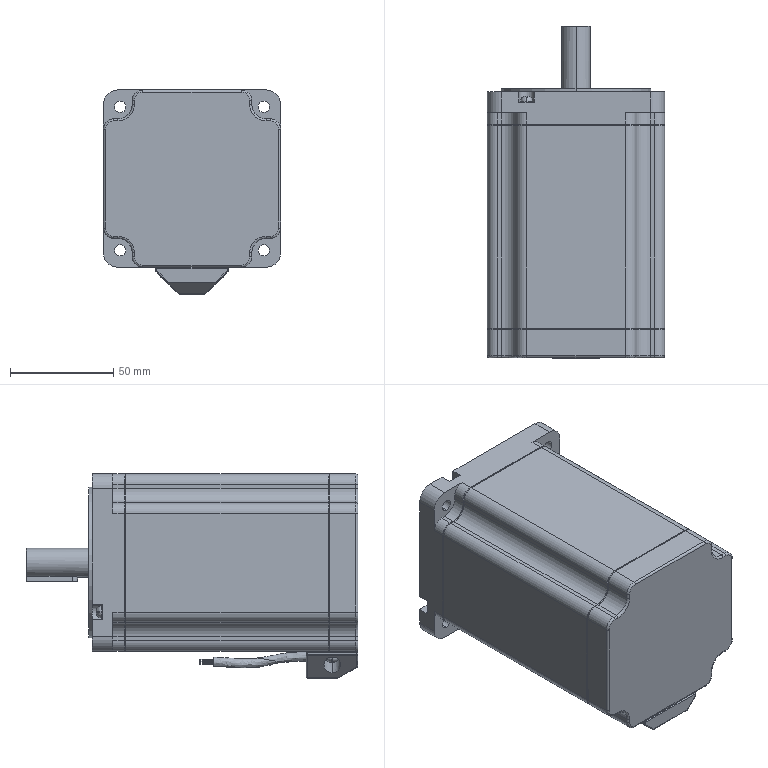Part | NX | features BREP 1 | 1 solid | 406 faces | box 86 x 161 x 99 mm | volume 875419 mm3 | plane 188 | cylinder 171 | torus 24 | sphere 20 | spline 2 | cone 1 | commonest cylinder face diameters 10 x40 6 x26 1 x20 14 x18 2 x12 0.4 x8